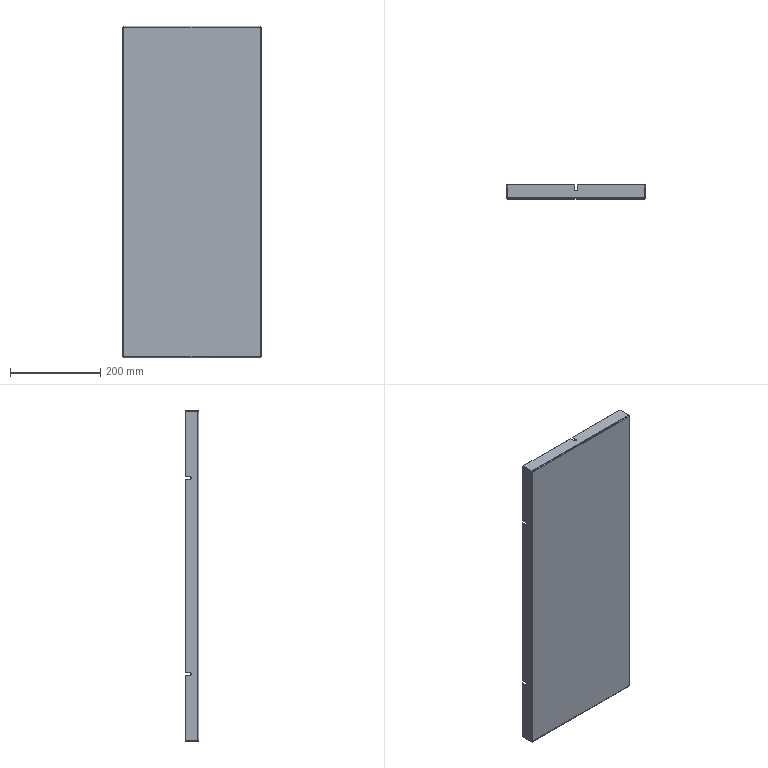Part | STEP file | JBJ-P-1000-10 | 1 solid | 62 faces | box 308 x 30 x 735 mm | volume 340907 mm3 | plane 40 | cylinder 14 | spline 8 | commonest cylinder face diameters 6.5 x6 2 x4 4.4 x4